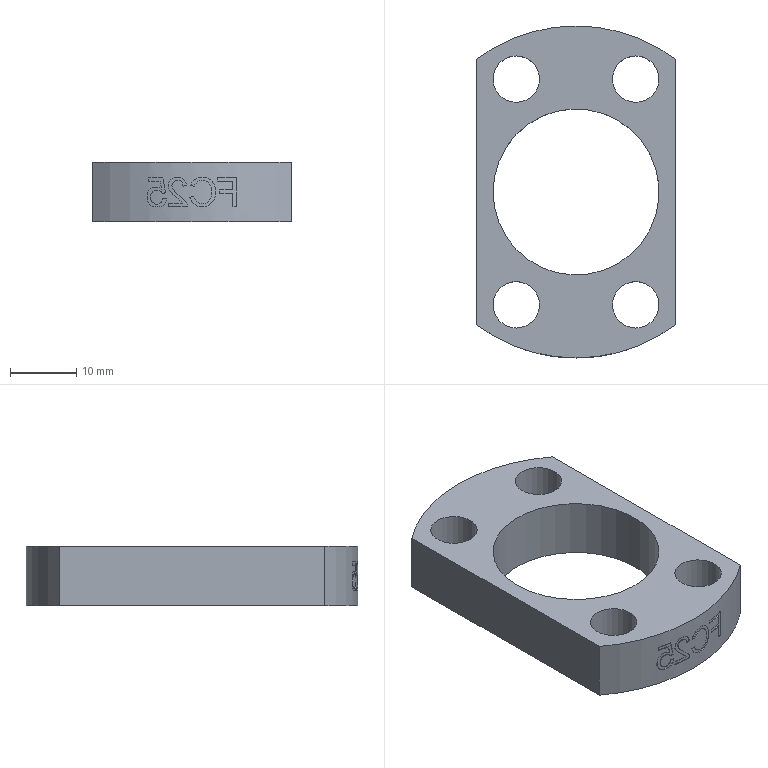Part | NX | features FC25_1 2 | 1 solid | 61 faces | box 30 x 50 x 9 mm | volume 6834 mm3 | plane 35 | cylinder 26 | commonest cylinder face diameters 7 x4 49.8 x4 50 x2 1.677 x1 1.765 x1 1.864 x1